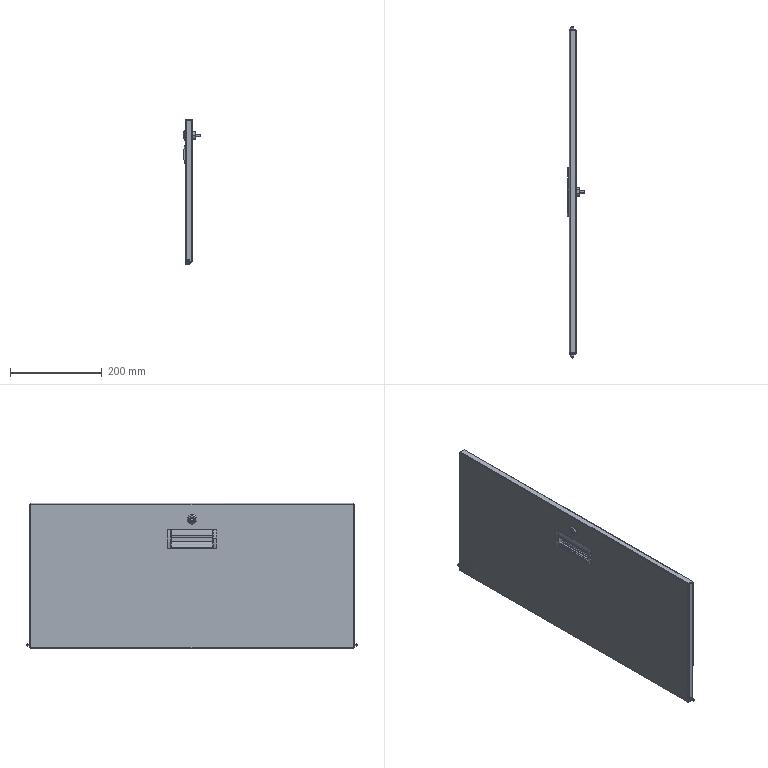Part | SolidWorks | 9 solids | 275 faces | box 37.5 x 724 x 317 mm | volume 427850 mm3 | plane 151 | cylinder 106 | spline 8 | cone 6 | torus 4 | commonest cylinder face diameters 1 x18 7 x10 5.5 x8 6 x8 0.6 x7 3.6 x7